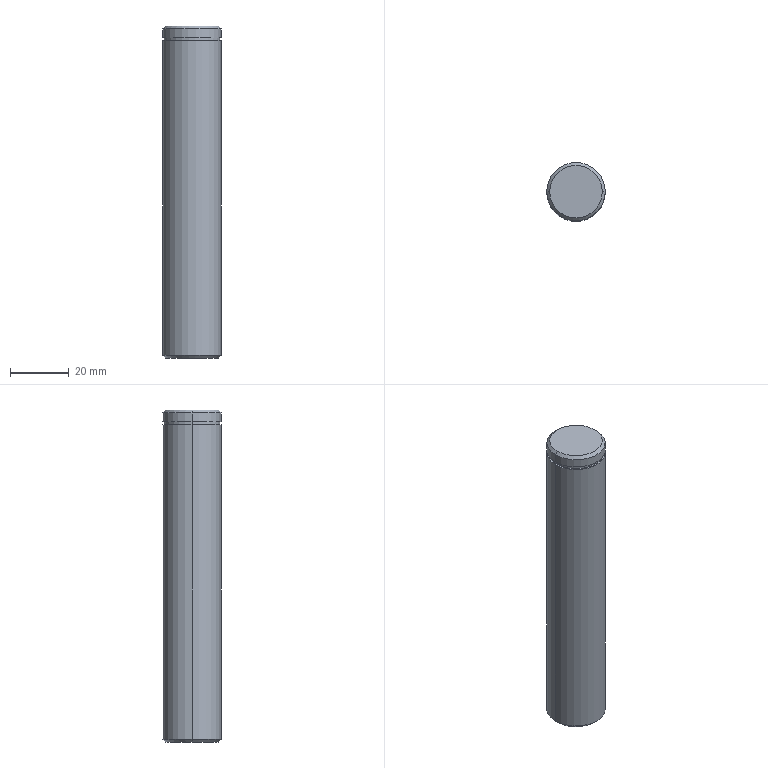Part | SolidWorks | features Chamfer 1, Extrusion 1, HoleWzd 1, RevCut 1 | 1 solid | 17 faces | box 20 x 20 x 113.5 mm | volume 35150 mm3 | cylinder 8 | plane 5 | cone 4 | commonest cylinder face diameters 20 x4 5 x2 19 x2
STEP:
#1=CARTESIAN_POINT('',(2.5,0.,21.));
#2=VERTEX_POINT('',#1);
#3=CARTESIAN_POINT('',(-2.5,0.,21.));
#4=VERTEX_POINT('',#3);
#5=CARTESIAN_POINT('',(0.,0.,21.));
#6=DIRECTION('',(0.,0.,-1.));
#7=DIRECTION('',(-1.,0.,0.));
#8=AXIS2_PLACEMENT_3D('',#5,#6,#7);
#9=CIRCLE('',#8,2.5);
#10=EDGE_CURVE('',#2,#4,#9,.T.);
#11=ORIENTED_EDGE('',*,*,#10,.F.);
#12=CARTESIAN_POINT('',(2.5,0.,0.));
#13=VERTEX_POINT('',#12);
#14=CARTESIAN_POINT('',(2.5,0.,0.));
#15=DIRECTION('',(0.,0.,-1.));
#16=VECTOR('',#15,1000.);
#17=LINE('',#14,#16);
#18=EDGE_CURVE('',#2,#13,#17,.T.);
#19=ORIENTED_EDGE('',*,*,#18,.T.);
#20=CARTESIAN_POINT('',(-2.5,0.,0.));
#21=VERTEX_POINT('',#20);
#22=CARTESIAN_POINT('',(0.,0.,0.));
#23=DIRECTION('',(0.,0.,-1.));
#24=DIRECTION('',(-1.,0.,0.));
#25=AXIS2_PLACEMENT_3D('',#22,#23,#24);
#26=CIRCLE('',#25,2.5);
#27=EDGE_CURVE('',#13,#21,#26,.T.);
#28=ORIENTED_EDGE('',*,*,#27,.T.);
#29=CARTESIAN_POINT('',(-2.5,0.,0.));
#30=DIRECTION('',(0.,0.,-1.));
#31=VECTOR('',#30,1000.);
#32=LINE('',#29,#31);
#33=EDGE_CURVE('',#4,#21,#32,.T.);
#34=ORIENTED_EDGE('',*,*,#33,.F.);
#35=EDGE_LOOP('',(#11,#19,#28,#34));
#36=FACE_OUTER_BOUND('',#35,.T.);
#37=CARTESIAN_POINT('',(0.,0.,0.));
#38=DIRECTION('',(0.,0.,-1.));
#39=DIRECTION('',(-1.,0.,0.));
#40=AXIS2_PLACEMENT_3D('',#37,#38,#39);
#41=CYLINDRICAL_SURFACE('',#40,2.5);
#42=ADVANCED_FACE('',(#36),#41,.F.);
#43=CARTESIAN_POINT('',(9.,0.,113.5));
#44=VERTEX_POINT('',#43);
#45=CARTESIAN_POINT('',(-9.,0.,113.5));
#46=VERTEX_POINT('',#45);
#47=CARTESIAN_POINT('',(0.,0.,113.5));
#48=DIRECTION('',(0.,0.,1.));
#49=DIRECTION('',(1.,0.,0.));
#50=AXIS2_PLACEMENT_3D('',#47,#48,#49);
#51=CIRCLE('',#50,9.);
#52=EDGE_CURVE('',#44,#46,#51,.T.);
#53=ORIENTED_EDGE('',*,*,#52,.F.);
#54=CARTESIAN_POINT('',(10.,0.,112.5));
#55=VERTEX_POINT('',#54);
#56=CARTESIAN_POINT('',(9.,0.,113.5));
#57=DIRECTION('',(0.7071,0.,-0.7071));
#58=VECTOR('',#57,1000.);
#59=LINE('',#56,#58);
#60=EDGE_CURVE('',#44,#55,#59,.T.);
#61=ORIENTED_EDGE('',*,*,#60,.T.);
#62=CARTESIAN_POINT('',(-10.,0.,112.5));
#63=VERTEX_POINT('',#62);
#64=CARTESIAN_POINT('',(0.,0.,112.5));
#65=DIRECTION('',(0.,0.,-1.));
#66=DIRECTION('',(1.,0.,0.));
#67=AXIS2_PLACEMENT_3D('',#64,#65,#66);
#68=CIRCLE('',#67,10.);
#69=EDGE_CURVE('',#63,#55,#68,.T.);
#70=ORIENTED_EDGE('',*,*,#69,.F.);
#71=CARTESIAN_POINT('',(-9.,0.,113.5));
#72=DIRECTION('',(-0.7071,0.,-0.7071));
#73=VECTOR('',#72,1000.);
#74=LINE('',#71,#73);
#75=EDGE_CURVE('',#46,#63,#74,.T.);
#76=ORIENTED_EDGE('',*,*,#75,.F.);
#77=EDGE_LOOP('',(#53,#61,#70,#76));
#78=FACE_OUTER_BOUND('',#77,.T.);
#79=CARTESIAN_POINT('',(0.,0.,113.5));
#80=DIRECTION('',(0.,0.,-1.));
#81=DIRECTION('',(-1.,0.,0.));
#82=AXIS2_PLACEMENT_3D('',#79,#80,#81);
#83=CONICAL_SURFACE('',#82,9.,0.7854);
#84=ADVANCED_FACE('',(#78),#83,.T.);
#85=CARTESIAN_POINT('',(-9.,0.,0.));
#86=VERTEX_POINT('',#85);
#87=CARTESIAN_POINT('',(9.,0.,0.));
#88=VERTEX_POINT('',#87);
#89=CARTESIAN_POINT('',(0.,0.,0.));
#90=DIRECTION('',(0.,0.,-1.));
#91=DIRECTION('',(1.,0.,0.));
#92=AXIS2_PLACEMENT_3D('',#89,#90,#91);
#93=CIRCLE('',#92,9.);
#94=EDGE_CURVE('',#86,#88,#93,.T.);
#95=ORIENTED_EDGE('',*,*,#94,.F.);
#96=CARTESIAN_POINT('',(-10.,0.,1.));
#97=VERTEX_POINT('',#96);
#98=CARTESIAN_POINT('',(-10.,0.,1.));
#99=DIRECTION('',(-0.7071,0.,0.7071));
#100=VECTOR('',#99,1000.);
#101=LINE('',#98,#100);
#102=EDGE_CURVE('',#86,#97,#101,.T.);
#103=ORIENTED_EDGE('',*,*,#102,.T.);
#104=CARTESIAN_POINT('',(10.,0.,1.));
#105=VERTEX_POINT('',#104);
#106=CARTESIAN_POINT('',(0.,0.,1.));
#107=DIRECTION('',(0.,0.,1.));
#108=DIRECTION('',(1.,0.,0.));
#109=AXIS2_PLACEMENT_3D('',#106,#107,#108);
#110=CIRCLE('',#109,10.);
#111=EDGE_CURVE('',#105,#97,#110,.T.);
#112=ORIENTED_EDGE('',*,*,#111,.F.);
#113=CARTESIAN_POINT('',(10.,0.,1.));
#114=DIRECTION('',(0.7071,0.,0.7071));
#115=VECTOR('',#114,1000.);
#116=LINE('',#113,#115);
#117=EDGE_CURVE('',#88,#105,#116,.T.);
#118=ORIENTED_EDGE('',*,*,#117,.F.);
#119=EDGE_LOOP('',(#95,#103,#112,#118));
#120=FACE_OUTER_BOUND('',#119,.T.);
#121=CARTESIAN_POINT('',(0.,0.,1.));
#122=DIRECTION('',(0.,0.,1.));
#123=DIRECTION('',(1.,0.,0.));
#124=AXIS2_PLACEMENT_3D('',#121,#122,#123);
#125=CONICAL_SURFACE('',#124,10.,0.7854);
#126=ADVANCED_FACE('',(#120),#125,.T.);
#127=CARTESIAN_POINT('',(10.,0.,108.4));
#128=VERTEX_POINT('',#127);
#129=CARTESIAN_POINT('',(-10.,0.,108.4));
#130=VERTEX_POINT('',#129);
#131=CARTESIAN_POINT('',(0.,0.,108.4));
#132=DIRECTION('',(0.,0.,1.));
#133=DIRECTION('',(1.,0.,0.));
#134=AXIS2_PLACEMENT_3D('',#131,#132,#133);
#135=CIRCLE('',#134,10.);
#136=EDGE_CURVE('',#128,#130,#135,.T.);
#137=ORIENTED_EDGE('',*,*,#136,.F.);
#138=CARTESIAN_POINT('',(10.,0.,113.5));
#139=DIRECTION('',(0.,0.,-1.));
#140=VECTOR('',#139,1000.);
#141=LINE('',#138,#140);
#142=EDGE_CURVE('',#128,#105,#141,.T.);
#143=ORIENTED_EDGE('',*,*,#142,.T.);
#144=ORIENTED_EDGE('',*,*,#111,.T.);
#145=CARTESIAN_POINT('',(-10.,0.,113.5));
#146=DIRECTION('',(0.,0.,-1.));
#147=VECTOR('',#146,1000.);
#148=LINE('',#145,#147);
#149=EDGE_CURVE('',#130,#97,#148,.T.);
#150=ORIENTED_EDGE('',*,*,#149,.F.);
#151=EDGE_LOOP('',(#137,#143,#144,#150));
#152=FACE_OUTER_BOUND('',#151,.T.);
#153=CARTESIAN_POINT('',(0.,0.,113.5));
#154=DIRECTION('',(0.,0.,-1.));
#155=DIRECTION('',(-1.,0.,0.));
#156=AXIS2_PLACEMENT_3D('',#153,#154,#155);
#157=CYLINDRICAL_SURFACE('',#156,10.);
#158=ADVANCED_FACE('',(#152),#157,.T.);
#159=CARTESIAN_POINT('',(9.5,0.,108.4));
#160=VERTEX_POINT('',#159);
#161=CARTESIAN_POINT('',(-9.5,0.,108.4));
#162=VERTEX_POINT('',#161);
#163=CARTESIAN_POINT('',(0.,0.,108.4));
#164=DIRECTION('',(0.,0.,1.));
#165=DIRECTION('',(1.,0.,0.));
#166=AXIS2_PLACEMENT_3D('',#163,#164,#165);
#167=CIRCLE('',#166,9.5);
#168=EDGE_CURVE('',#160,#162,#167,.T.);
#169=ORIENTED_EDGE('',*,*,#168,.T.);
#170=CARTESIAN_POINT('',(-9.5,0.,109.5));
#171=VERTEX_POINT('',#170);
#172=CARTESIAN_POINT('',(-9.5,0.,113.5));
#173=DIRECTION('',(0.,0.,1.));
#174=VECTOR('',#173,1000.);
#175=LINE('',#172,#174);
#176=EDGE_CURVE('',#162,#171,#175,.T.);
#177=ORIENTED_EDGE('',*,*,#176,.T.);
#178=CARTESIAN_POINT('',(9.5,0.,109.5));
#179=VERTEX_POINT('',#178);
#180=CARTESIAN_POINT('',(0.,0.,109.5));
#181=DIRECTION('',(0.,0.,1.));
#182=DIRECTION('',(1.,0.,0.));
#183=AXIS2_PLACEMENT_3D('',#180,#181,#182);
#184=CIRCLE('',#183,9.5);
#185=EDGE_CURVE('',#179,#171,#184,.T.);
#186=ORIENTED_EDGE('',*,*,#185,.F.);
#187=CARTESIAN_POINT('',(9.5,0.,113.5));
#188=DIRECTION('',(0.,0.,1.));
#189=VECTOR('',#188,1000.);
#190=LINE('',#187,#189);
#191=EDGE_CURVE('',#160,#179,#190,.T.);
#192=ORIENTED_EDGE('',*,*,#191,.F.);
#193=EDGE_LOOP('',(#169,#177,#186,#192));
#194=FACE_OUTER_BOUND('',#193,.T.);
#195=CARTESIAN_POINT('',(0.,0.,113.5));
#196=DIRECTION('',(0.,0.,1.));
#197=DIRECTION('',(1.,0.,0.));
#198=AXIS2_PLACEMENT_3D('',#195,#196,#197);
#199=CYLINDRICAL_SURFACE('',#198,9.5);
#200=ADVANCED_FACE('',(#194),#199,.T.);
#201=ORIENTED_EDGE('',*,*,#69,.T.);
#202=CARTESIAN_POINT('',(10.,0.,109.5));
#203=VERTEX_POINT('',#202);
#204=CARTESIAN_POINT('',(10.,0.,113.5));
#205=DIRECTION('',(0.,0.,-1.));
#206=VECTOR('',#205,1000.);
#207=LINE('',#204,#206);
#208=EDGE_CURVE('',#55,#203,#207,.T.);
#209=ORIENTED_EDGE('',*,*,#208,.T.);
#210=CARTESIAN_POINT('',(-10.,0.,109.5));
#211=VERTEX_POINT('',#210);
#212=CARTESIAN_POINT('',(0.,0.,109.5));
#213=DIRECTION('',(0.,0.,1.));
#214=DIRECTION('',(1.,0.,0.));
#215=AXIS2_PLACEMENT_3D('',#212,#213,#214);
#216=CIRCLE('',#215,10.);
#217=EDGE_CURVE('',#203,#211,#216,.T.);
#218=ORIENTED_EDGE('',*,*,#217,.T.);
#219=CARTESIAN_POINT('',(-10.,0.,113.5));
#220=DIRECTION('',(0.,0.,-1.));
#221=VECTOR('',#220,1000.);
#222=LINE('',#219,#221);
#223=EDGE_CURVE('',#63,#211,#222,.T.);
#224=ORIENTED_EDGE('',*,*,#223,.F.);
#225=EDGE_LOOP('',(#201,#209,#218,#224));
#226=FACE_OUTER_BOUND('',#225,.T.);
#227=CARTESIAN_POINT('',(0.,0.,113.5));
#228=DIRECTION('',(0.,0.,-1.));
#229=DIRECTION('',(-1.,0.,0.));
#230=AXIS2_PLACEMENT_3D('',#227,#228,#229);
#231=CYLINDRICAL_SURFACE('',#230,10.);
#232=ADVANCED_FACE('',(#226),#231,.T.);
#233=ORIENTED_EDGE('',*,*,#208,.F.);
#234=CARTESIAN_POINT('',(0.,0.,112.5));
#235=DIRECTION('',(0.,0.,-1.));
#236=DIRECTION('',(1.,0.,0.));
#237=AXIS2_PLACEMENT_3D('',#234,#235,#236);
#238=CIRCLE('',#237,10.);
#239=EDGE_CURVE('',#55,#63,#238,.T.);
#240=ORIENTED_EDGE('',*,*,#239,.T.);
#241=ORIENTED_EDGE('',*,*,#223,.T.);
#242=CARTESIAN_POINT('',(0.,0.,109.5));
#243=DIRECTION('',(0.,0.,1.));
#244=DIRECTION('',(1.,0.,0.));
#245=AXIS2_PLACEMENT_3D('',#242,#243,#244);
#246=CIRCLE('',#245,10.);
#247=EDGE_CURVE('',#211,#203,#246,.T.);
#248=ORIENTED_EDGE('',*,*,#247,.T.);
#249=EDGE_LOOP('',(#233,#240,#241,#248));
#250=FACE_OUTER_BOUND('',#249,.T.);
#251=CARTESIAN_POINT('',(0.,0.,113.5));
#252=DIRECTION('',(0.,0.,-1.));
#253=DIRECTION('',(-1.,0.,0.));
#254=AXIS2_PLACEMENT_3D('',#251,#252,#253);
#255=CYLINDRICAL_SURFACE('',#254,10.);
#256=ADVANCED_FACE('',(#250),#255,.T.);
#257=CARTESIAN_POINT('',(0.,0.,113.5));
#258=DIRECTION('',(0.,0.,1.));
#259=DIRECTION('',(1.,0.,0.));
#260=AXIS2_PLACEMENT_3D('',#257,#258,#259);
#261=CIRCLE('',#260,9.);
#262=EDGE_CURVE('',#46,#44,#261,.T.);
#263=ORIENTED_EDGE('',*,*,#262,.T.);
#264=ORIENTED_EDGE('',*,*,#52,.T.);
#265=EDGE_LOOP('',(#263,#264));
#266=FACE_OUTER_BOUND('',#265,.T.);
#267=CARTESIAN_POINT('',(0.,0.,113.5));
#268=DIRECTION('',(0.,0.,1.));
#269=DIRECTION('',(1.,0.,0.));
#270=AXIS2_PLACEMENT_3D('',#267,#268,#269);
#271=PLANE('',#270);
#272=ADVANCED_FACE('',(#266),#271,.T.);
#273=ORIENTED_EDGE('',*,*,#247,.F.);
#274=ORIENTED_EDGE('',*,*,#217,.F.);
#275=EDGE_LOOP('',(#273,#274));
#276=FACE_OUTER_BOUND('',#275,.T.);
#277=ORIENTED_EDGE('',*,*,#185,.T.);
#278=CARTESIAN_POINT('',(0.,0.,109.5));
#279=DIRECTION('',(0.,0.,1.));
#280=DIRECTION('',(1.,0.,0.));
#281=AXIS2_PLACEMENT_3D('',#278,#279,#280);
#282=CIRCLE('',#281,9.5);
#283=EDGE_CURVE('',#171,#179,#282,.T.);
#284=ORIENTED_EDGE('',*,*,#283,.T.);
#285=EDGE_LOOP('',(#277,#284));
#286=FACE_BOUND('',#285,.T.);
#287=CARTESIAN_POINT('',(10.,0.,109.5));
#288=DIRECTION('',(0.,0.,1.));
#289=DIRECTION('',(1.,0.,0.));
#290=AXIS2_PLACEMENT_3D('',#287,#288,#289);
#291=PLANE('',#290);
#292=ADVANCED_FACE('',(#276,#286),#291,.F.);
#293=ORIENTED_EDGE('',*,*,#176,.F.);
#294=CARTESIAN_POINT('',(0.,0.,108.4));
#295=DIRECTION('',(0.,0.,1.));
#296=DIRECTION('',(1.,0.,0.));
#297=AXIS2_PLACEMENT_3D('',#294,#295,#296);
#298=CIRCLE('',#297,9.5);
#299=EDGE_CURVE('',#162,#160,#298,.T.);
#300=ORIENTED_EDGE('',*,*,#299,.T.);
#301=ORIENTED_EDGE('',*,*,#191,.T.);
#302=ORIENTED_EDGE('',*,*,#283,.F.);
#303=EDGE_LOOP('',(#293,#300,#301,#302));
#304=FACE_OUTER_BOUND('',#303,.T.);
#305=CARTESIAN_POINT('',(0.,0.,113.5));
#306=DIRECTION('',(0.,0.,1.));
#307=DIRECTION('',(1.,0.,0.));
#308=AXIS2_PLACEMENT_3D('',#305,#306,#307);
#309=CYLINDRICAL_SURFACE('',#308,9.5);
#310=ADVANCED_FACE('',(#304),#309,.T.);
#311=ORIENTED_EDGE('',*,*,#168,.F.);
#312=ORIENTED_EDGE('',*,*,#299,.F.);
#313=EDGE_LOOP('',(#311,#312));
#314=FACE_BOUND('',#313,.T.);
#315=CARTESIAN_POINT('',(0.,0.,108.4));
#316=DIRECTION('',(0.,0.,1.));
#317=DIRECTION('',(1.,0.,0.));
#318=AXIS2_PLACEMENT_3D('',#315,#316,#317);
#319=CIRCLE('',#318,10.);
#320=EDGE_CURVE('',#130,#128,#319,.T.);
#321=ORIENTED_EDGE('',*,*,#320,.T.);
#322=ORIENTED_EDGE('',*,*,#136,.T.);
#323=EDGE_LOOP('',(#321,#322));
#324=FACE_OUTER_BOUND('',#323,.T.);
#325=CARTESIAN_POINT('',(10.,0.,108.4));
#326=DIRECTION('',(0.,0.,-1.));
#327=DIRECTION('',(-1.,0.,0.));
#328=AXIS2_PLACEMENT_3D('',#325,#326,#327);
#329=PLANE('',#328);
#330=ADVANCED_FACE('',(#314,#324),#329,.F.);
#331=CARTESIAN_POINT('',(0.,0.,0.));
#332=DIRECTION('',(0.,0.,-1.));
#333=DIRECTION('',(-1.,0.,0.));
#334=AXIS2_PLACEMENT_3D('',#331,#332,#333);
#335=CIRCLE('',#334,2.5);
#336=EDGE_CURVE('',#21,#13,#335,.T.);
#337=ORIENTED_EDGE('',*,*,#336,.F.);
#338=ORIENTED_EDGE('',*,*,#27,.F.);
#339=EDGE_LOOP('',(#337,#338));
#340=FACE_BOUND('',#339,.T.);
#341=CARTESIAN_POINT('',(0.,0.,0.));
#342=DIRECTION('',(0.,0.,-1.));
#343=DIRECTION('',(1.,0.,0.));
#344=AXIS2_PLACEMENT_3D('',#341,#342,#343);
#345=CIRCLE('',#344,9.);
#346=EDGE_CURVE('',#88,#86,#345,.T.);
#347=ORIENTED_EDGE('',*,*,#346,.T.);
#348=ORIENTED_EDGE('',*,*,#94,.T.);
#349=EDGE_LOOP('',(#347,#348));
#350=FACE_OUTER_BOUND('',#349,.T.);
#351=CARTESIAN_POINT('',(0.,0.,0.));
#352=DIRECTION('',(0.,0.,1.));
#353=DIRECTION('',(1.,0.,0.));
#354=AXIS2_PLACEMENT_3D('',#351,#352,#353);
#355=PLANE('',#354);
#356=ADVANCED_FACE('',(#340,#350),#355,.F.);
#357=ORIENTED_EDGE('',*,*,#142,.F.);
#358=ORIENTED_EDGE('',*,*,#320,.F.);
#359=ORIENTED_EDGE('',*,*,#149,.T.);
#360=CARTESIAN_POINT('',(0.,0.,1.));
#361=DIRECTION('',(0.,0.,1.));
#362=DIRECTION('',(1.,0.,0.));
#363=AXIS2_PLACEMENT_3D('',#360,#361,#362);
#364=CIRCLE('',#363,10.);
#365=EDGE_CURVE('',#97,#105,#364,.T.);
#366=ORIENTED_EDGE('',*,*,#365,.T.);
#367=EDGE_LOOP('',(#357,#358,#359,#366));
#368=FACE_OUTER_BOUND('',#367,.T.);
#369=CARTESIAN_POINT('',(0.,0.,113.5));
#370=DIRECTION('',(0.,0.,-1.));
#371=DIRECTION('',(-1.,0.,0.));
#372=AXIS2_PLACEMENT_3D('',#369,#370,#371);
#373=CYLINDRICAL_SURFACE('',#372,10.);
#374=ADVANCED_FACE('',(#368),#373,.T.);
#375=ORIENTED_EDGE('',*,*,#102,.F.);
#376=ORIENTED_EDGE('',*,*,#346,.F.);
#377=ORIENTED_EDGE('',*,*,#117,.T.);
#378=ORIENTED_EDGE('',*,*,#365,.F.);
#379=EDGE_LOOP('',(#375,#376,#377,#378));
#380=FACE_OUTER_BOUND('',#379,.T.);
#381=CARTESIAN_POINT('',(0.,0.,1.));
#382=DIRECTION('',(0.,0.,1.));
#383=DIRECTION('',(1.,0.,0.));
#384=AXIS2_PLACEMENT_3D('',#381,#382,#383);
#385=CONICAL_SURFACE('',#384,10.,0.7854);
#386=ADVANCED_FACE('',(#380),#385,.T.);
#387=ORIENTED_EDGE('',*,*,#60,.F.);
#388=ORIENTED_EDGE('',*,*,#262,.F.);
#389=ORIENTED_EDGE('',*,*,#75,.T.);
#390=ORIENTED_EDGE('',*,*,#239,.F.);
#391=EDGE_LOOP('',(#387,#388,#389,#390));
#392=FACE_OUTER_BOUND('',#391,.T.);
#393=CARTESIAN_POINT('',(0.,0.,113.5));
#394=DIRECTION('',(0.,0.,-1.));
#395=DIRECTION('',(-1.,0.,0.));
#396=AXIS2_PLACEMENT_3D('',#393,#394,#395);
#397=CONICAL_SURFACE('',#396,9.,0.7854);
#398=ADVANCED_FACE('',(#392),#397,.T.);
#399=CARTESIAN_POINT('',(0.,0.,21.));
#400=DIRECTION('',(0.,0.,-1.));
#401=DIRECTION('',(-1.,0.,0.));
#402=AXIS2_PLACEMENT_3D('',#399,#400,#401);
#403=CIRCLE('',#402,2.5);
#404=EDGE_CURVE('',#4,#2,#403,.T.);
#405=ORIENTED_EDGE('',*,*,#404,.T.);
#406=ORIENTED_EDGE('',*,*,#10,.T.);
#407=EDGE_LOOP('',(#405,#406));
#408=FACE_OUTER_BOUND('',#407,.T.);
#409=CARTESIAN_POINT('',(0.,0.,21.));
#410=DIRECTION('',(0.,0.,1.));
#411=DIRECTION('',(1.,0.,0.));
#412=AXIS2_PLACEMENT_3D('',#409,#410,#411);
#413=PLANE('',#412);
#414=ADVANCED_FACE('',(#408),#413,.F.);
#415=ORIENTED_EDGE('',*,*,#18,.F.);
#416=ORIENTED_EDGE('',*,*,#404,.F.);
#417=ORIENTED_EDGE('',*,*,#33,.T.);
#418=ORIENTED_EDGE('',*,*,#336,.T.);
#419=EDGE_LOOP('',(#415,#416,#417,#418));
#420=FACE_OUTER_BOUND('',#419,.T.);
#421=CARTESIAN_POINT('',(0.,0.,0.));
#422=DIRECTION('',(0.,0.,-1.));
#423=DIRECTION('',(-1.,0.,0.));
#424=AXIS2_PLACEMENT_3D('',#421,#422,#423);
#425=CYLINDRICAL_SURFACE('',#424,2.5);
#426=ADVANCED_FACE('',(#420),#425,.F.);
#427=CLOSED_SHELL('',(#42,#84,#126,#158,#200,#232,#256,#272,#292,#310,#330,#356,#374,#386,#398,#414,#426));
#428=MANIFOLD_SOLID_BREP('',#427);
#429=CARTESIAN_POINT('',(0.,0.,0.));
#430=DIRECTION('',(0.,0.,1.));
#431=DIRECTION('',(1.,0.,0.));
#432=AXIS2_PLACEMENT_3D('',#429,#430,#431);
#433=(LENGTH_UNIT()NAMED_UNIT(*)SI_UNIT(.MILLI.,.METRE.));
#434=UNCERTAINTY_MEASURE_WITH_UNIT(LENGTH_MEASURE(0.00001),#433,'','');
#435=(NAMED_UNIT(*)PLANE_ANGLE_UNIT()SI_UNIT($,.RADIAN.));
#436=(NAMED_UNIT(*)SI_UNIT($,.STERADIAN.)SOLID_ANGLE_UNIT());
#437=(GEOMETRIC_REPRESENTATION_CONTEXT(3)GLOBAL_UNCERTAINTY_ASSIGNED_CONTEXT((#434))GLOBAL_UNIT_ASSIGNED_CONTEXT((#433,#435,#436))REPRESENTATION_CONTEXT('',''));
#438=ADVANCED_BREP_SHAPE_REPRESENTATION('',(#428,#432),#437);